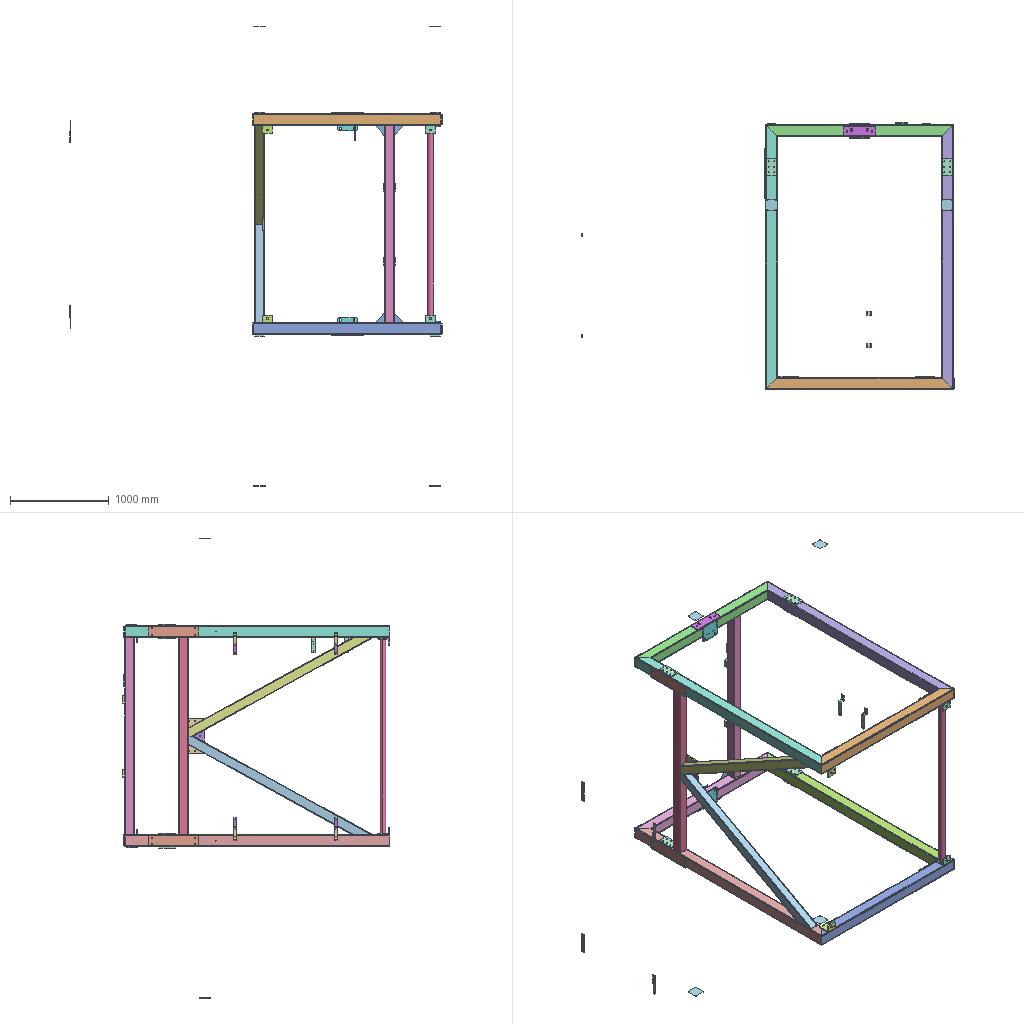Assembly | SolidWorks | 34 different items | 72 placed | box 3771 x 2705 x 4658 mm
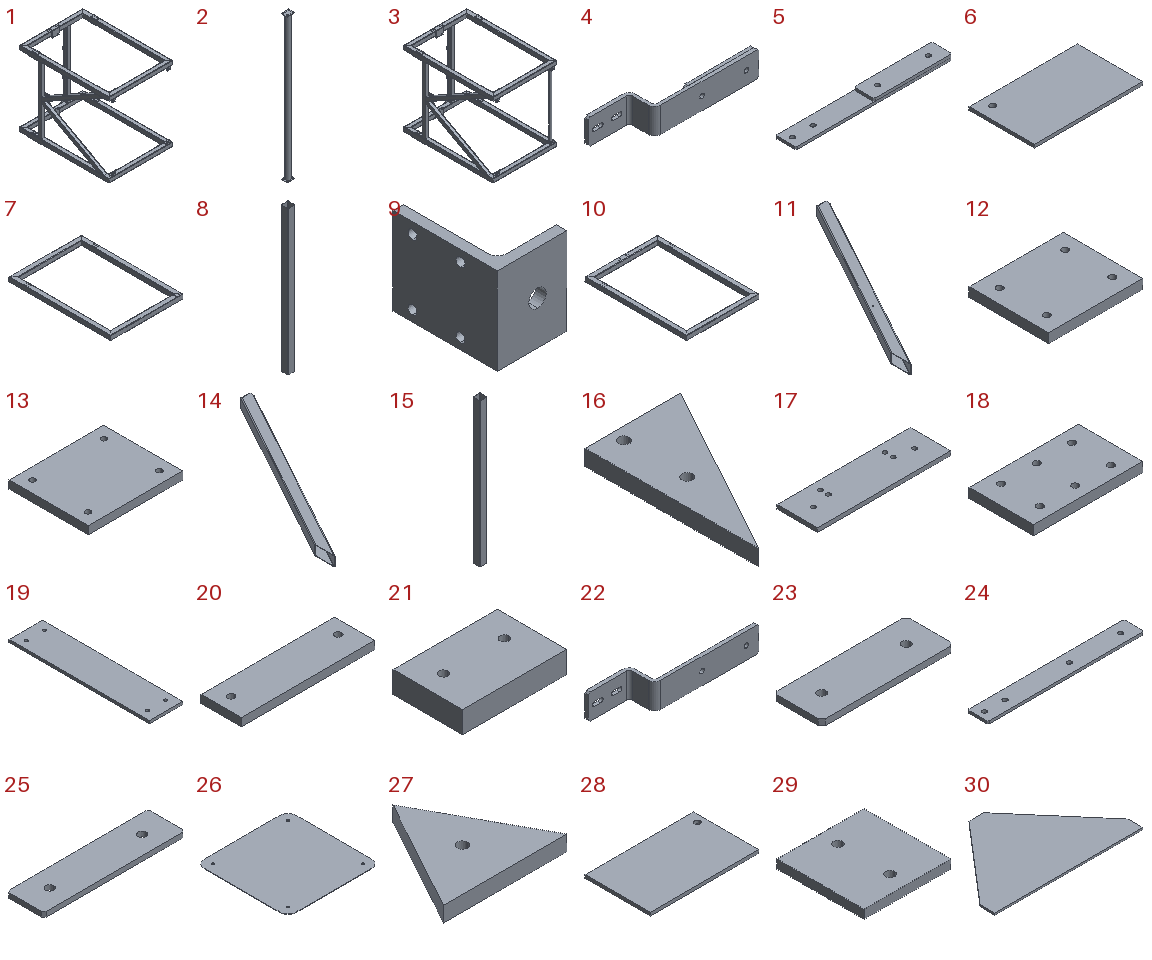Parts list (item | name | quantity | parent item | size | volume | features):
1 | (subassembly) | x1 | in 3 | 1920 x 2705 x 2270 mm | 51706109 mm3 | features CompositeCurve 25
2 | (subassembly) | x1 | in 3 | 100 x 80 x 1976 mm | 1280209 mm3 | -
3 | (subassembly) | x1 | - | 1920 x 2705 x 2270 mm | 52986318 mm3 | features CompositeCurve 4
4 | (subassembly) | x2 | - | 230 x 45 x 40 mm | 72678 mm3 | -
5 | (subassembly) | x4 | - | 230 x 30 x 8 mm | 40540 mm3 | features CompositeCurve 1
6 | - | x2 | in 1 | 200 x 120 x 6 mm | 143510 mm3 | features Extrusion 1, HoleWzd 1
7 | - | x1 | in 1 | 1900 x 2680 x 120 mm | 15591720 mm3 | features ICE 8, HoleWzd 6, 3DProfileFeature 1, WeldMemberFeat 1, WeldmentFeature 1
8 | - | x1 | in 1 | 100 x 100 x 2000 mm | 2980690 mm3 | features Extrusion 1, Fillet 1, HoleWzd 1, ICE 1, Shell 1
9 | - | x2 | in 1 | 80 x 120 x 100 mm | 220054 mm3 | features Extrusion 1, HoleWzd 1, ICE 1
10 | - | x1 | in 1 | 1900 x 2680 x 120 mm | 15602458 mm3 | features HoleWzd 7, ICE 7, WeldMemberFeat 1, WeldmentFeature 1
11 | - | x1 | in 1 | 1000 x 1874 x 100 mm | 3026106 mm3 | features Fillet 2, Extrusion 1, HoleWzd 1, Shell 1
12 | - | x4 | in 1 | 100 x 85 x 10 mm | 83547 mm3 | features Extrusion 1, HoleWzd 1
13 | - | x1 | in 1 | 120 x 100 x 10 mm | 118547 mm3 | features Extrusion 1, HoleWzd 1
14 | - | x1 | in 1 | 1000 x 1874 x 100 mm | 3026106 mm3 | features Fillet 2, Extrusion 1, HoleWzd 1, Shell 1
15 | - | x1 | in 1 | 100 x 100 x 2000 mm | 2986846 mm3 | features Extrusion 1, Shell 1
16 | - | x2 | in 1 | 90.635 x 165 x 15 mm | 109709 mm3 | features Extrusion 1, HoleWzd 1
17 | - | x2 | in 1 | 330 x 100 x 10 mm | 325097 mm3 | features Extrusion 1, HoleWzd 1
18 | - | x8 | in 1 | 170 x 100 x 15 mm | 247646 mm3 | features Extrusion 1, HoleWzd 1
19 | - | x2 | in 1 | 120 x 505 x 10 mm | 602731 mm3 | features Extrusion 1, HoleWzd 1
20 | - | x2 | in 1 | 200 x 60 x 12 mm | 142039 mm3 | features Extrusion 1, HoleWzd 1
21 | - | x2 | in 1 | 120 x 80 x 25 mm | 235914 mm3 | features Extrusion 1, HoleWzd 1
22 | - | x2 | in 4 | 230 x 45 x 40 mm | 51153 mm3 | features ICE 2, Chamfer 1, Extrusion 1
23 | - | x2 | in 4 | 110 x 40 x 5 mm | 21525 mm3 | features Chamfer 1, Extrusion 1
24 | - | x4 | in 5 | 230 x 30 x 4 mm | 27037 mm3 | features Chamfer 1, Extrusion 1
25 | - | x4 | in 5 | 115 x 30 x 4 mm | 13503 mm3 | features Chamfer 1, Extrusion 1
26 | - | x4 | - | 115 x 115 x 0.5 mm | 6555 mm3 | features Extrusion 1
27 | - | x1 | in 1 | 121 x 110.14 x 15 mm | 98726 mm3 | features Extrusion 1, HoleWzd 1
28 | - | x2 | in 1 | 200 x 120 x 6 mm | 143510 mm3 | features Extrusion 1, HoleWzd 1
29 | - | x2 | in 1 | 100 x 100 x 10 mm | 98366 mm3 | features Extrusion 1, HoleWzd 1
30 | - | x2 | in 1 | 400 x 250 x 5 mm | 311000 mm3 | features Extrusion 1, ICE 1
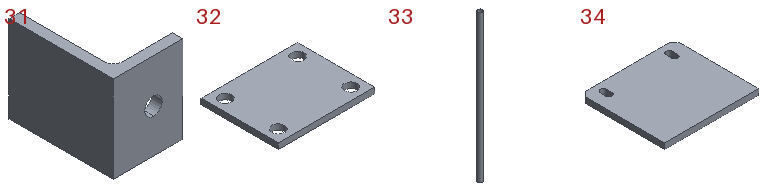31 | - | x2 | in 1 | 80 x 120 x 100 mm | 223976 mm3 | features Extrusion 1, ICE 1
32 | - | x2 | in 2 | 100 x 80 x 6 mm | 44814 mm3 | features Extrusion 1, ICE 1
33 | - | x1 | in 2 | 63.5 x 63.5 x 1964 mm | 1190580 mm3 | features Extrusion 1, Shell 1
34 | - | x2 | in 1 | 200 x 180 x 12 mm | 423870 mm3 | features Chamfer 1, Extrusion 1, ICE 1
Mates (type | each side: item.copy, entity, surface, feature):
In the top assembly
Coincident | 7.1 face plane Rectangular Tube 120 X 80 X 8(1) | 26.1 face plane Boss-Extrude1
Concentric | 7.1 edge | 26.1 edge
Coincident | 7.1 face cylinder Cut-Extrude1 | 26.1 edge
Coincident | 26.2 face plane Boss-Extrude1 | 26.1 face plane Boss-Extrude1
Coincident | 7.1 face cylinder Cut-Extrude1 | 26.2 edge
Concentric | 7.1 face cylinder Cut-Extrude1 | 26.2 face cylinder Boss-Extrude1
Coincident | 10.1 face plane Rectangular Tube 120 X 80 X 8(1) | 26.3 face plane Boss-Extrude1
Coincident | 10.1 face plane Rectangular Tube 120 X 80 X 8(1) | 26.4 face plane Boss-Extrude1
Concentric | 10.1 face cylinder Cut-Extrude5 | 26.4 face cylinder Boss-Extrude1 | 2 times
Concentric | 10.1 face cylinder Cut-Extrude5 | 26.3 face cylinder Boss-Extrude1 | 2 times
Coincident | 10.1 face plane Rectangular Tube 120 X 80 X 8(1) | 24.1 face plane Boss-Extrude1
Concentric | 10.1 edge | 24.1 edge | 2 times
Coincident | 10.1 face plane Rectangular Tube 120 X 80 X 8(1) | 24.2 face plane Boss-Extrude1
Concentric | 10.1 face cylinder M6 Tapped Hole1 | 24.2 face cylinder Boss-Extrude1 | 2 times
Coincident | 7.1 face plane Rectangular Tube 120 X 80 X 8(1) | 24.3 face plane Boss-Extrude1
Concentric | 7.1 face cylinder M6 Tapped Hole1 | 24.3 edge
Concentric | 7.1 face cylinder M6 Tapped Hole1 | 24.3 face cylinder Boss-Extrude1
Coincident | 7.1 face plane Rectangular Tube 120 X 80 X 8(1) | 24.4 face plane Boss-Extrude1
Concentric | 7.1 face cylinder M6 Tapped Hole1 | 24.4 face cylinder Boss-Extrude1
Concentric | 7.1 edge | 24.4 face cylinder Boss-Extrude1
Coincident | 10.1 face plane Rectangular Tube 120 X 80 X 8(1) | 22.1 face plane Boss-Extrude1
Parallel | 10.1 face plane Rectangular Tube 120 X 80 X 8(1) | 22.1 face plane Boss-Extrude1
Coincident | 10.1 face plane Rectangular Tube 120 X 80 X 8(1) | 22.2 face plane Boss-Extrude1
Coincident | 22.1 face plane Boss-Extrude1 | 22.2 face plane Boss-Extrude1
In subassembly 4
Coincident | 22.3 face plane Boss-Extrude1 | 23.1 face plane Boss-Extrude1
Concentric | 22.3 face cylinder Cut-Extrude2 | 23.1 face cylinder Boss-Extrude1 | 2 times
In subassembly 5
Coincident | 24.5 face plane Boss-Extrude1 | 25.1 face plane Boss-Extrude1
Coincident | 24.5 edge | 25.1 face cylinder Boss-Extrude1
Concentric | 24.5 face cylinder Boss-Extrude1 | 25.1 face cylinder Boss-Extrude1
In subassembly 3
Coincident | 9.1 face plane Boss-Extrude1 | 32.1 face plane Boss-Extrude1
Concentric | 9.1 select_type:24 | 32.1 edge
Concentric | 9.1 edge | 32.1 edge
In subassembly 2
Coincident | 32.2 face plane Boss-Extrude1 | 33.1 face plane Boss-Extrude1
Coincident | 32.2 plane | 33.1 plane | 2 times
Coincident | 32.2 face plane Boss-Extrude1 | 32.3 face plane Boss-Extrude1 | 2 times
Coincident | 33.1 face plane Boss-Extrude1 | 32.3 face plane Boss-Extrude1
In subassembly 1
Coincident | 7.2 face plane Rectangular Tube 120 X 80 X 8(1) | 10.2 face plane Rectangular Tube 120 X 80 X 8(1) | 2 times
Coincident | 7.2 face plane Rectangular Tube 120 X 80 X 8(1) | 15.1 face plane Boss-Extrude1
Coincident | 10.2 face plane Rectangular Tube 120 X 80 X 8(1) | 15.1 face plane Boss-Extrude1
DistanceDim | 15.1 face plane Boss-Extrude1 | 7.2 face plane Rectangular Tube 120 X 80 X 8(1)
Width | 7.2 face plane Rectangular Tube 120 X 80 X 8(1) | 7.2 face plane Rectangular Tube 120 X 80 X 8(1) | 15.1 face plane Boss-Extrude1 | 15.1 face plane Boss-Extrude1
Coincident | 7.2 face plane Rectangular Tube 120 X 80 X 8(1) | 14.1 face plane Boss-Extrude1
Width | 14.1 face plane Boss-Extrude1 | 14.1 face plane Boss-Extrude1 | 7.2 face plane Rectangular Tube 120 X 80 X 8(1) | 7.2 face plane Rectangular Tube 120 X 80 X 8(1)
Coincident | 15.1 face plane Boss-Extrude1 | 14.1 face plane Boss-Extrude1
Coincident | 10.2 face plane Rectangular Tube 120 X 80 X 8(1) | 11.1 face plane Boss-Extrude1
Coincident | 14.1 face plane Boss-Extrude1 | 11.1 face plane Boss-Extrude1 | 2 times
Coincident | 15.1 face plane Boss-Extrude1 | 11.1 face plane Boss-Extrude1
Coincident | 10.2 face plane Rectangular Tube 120 X 80 X 8(1) | 17.1 face plane Boss-Extrude1
Concentric | 10.2 edge | 17.1 edge | 2 times
Coincident | 7.2 face plane Rectangular Tube 120 X 80 X 8(1) | 17.2 face plane Boss-Extrude1
Concentric | 7.2 edge | 17.2 face cylinder M12 Tapped Hole1
Concentric | 7.2 edge | 17.2 edge
Coincident | 7.2 face plane Rectangular Tube 120 X 80 X 8(1) | 18.1 face plane Boss-Extrude1
Concentric | 7.2 edge | 18.1 edge | 2 times
Coincident | 7.2 face plane Rectangular Tube 120 X 80 X 8(1) | 18.2 face plane Boss-Extrude1
Concentric | 7.2 edge | 18.2 edge | 2 times
Concentric | 7.2 face cylinder Cut-Extrude2 | 18.3 face cylinder M12 Tapped Hole1 | 2 times
Coincident | 7.2 face plane Rectangular Tube 120 X 80 X 8(1) | 18.3 face plane Boss-Extrude1
Coincident | 7.2 face plane Rectangular Tube 120 X 80 X 8(1) | 18.4 face plane Boss-Extrude1
Concentric | 7.2 edge | 19.1 edge | 2 times
Coincident | 19.1 face plane Boss-Extrude1 | 19.2 face plane Boss-Extrude1
Concentric | 10.2 face cylinder M12 Tapped Hole1 | 19.2 face cylinder M12 Tapped Hole1 | 2 times
Coincident | 7.2 face plane Rectangular Tube 120 X 80 X 8(1) | 19.1 face plane Boss-Extrude1
Coincident | 7.2 face plane Rectangular Tube 120 X 80 X 8(1) | 20.1 face plane Boss-Extrude1
Concentric | 7.2 face cylinder Cut-Extrude10 | 20.1 face cylinder M12 Tapped Hole1 | 2 times
Coincident | 10.2 face plane Rectangular Tube 120 X 80 X 8(1) | 20.2 face plane Boss-Extrude1
Concentric | 10.2 face cylinder Cut-Extrude7 | 20.2 face cylinder M12 Tapped Hole1 | 2 times
Coincident | 7.2 face plane Rectangular Tube 120 X 80 X 8(1) | 8.1 face plane Boss-Extrude1 | 2 times
DistanceDim | 8.1 face plane Boss-Extrude1 | 10.2 face plane Rectangular Tube 120 X 80 X 8(1)
Coincident | 21.1 face plane Boss-Extrude1 | 21.2 face plane Boss-Extrude1
Coincident | 21.2 face plane Boss-Extrude1 | 8.1 face plane Boss-Extrude1
Coincident | 10.2 face plane Rectangular Tube 120 X 80 X 8(1) | 34.1 face plane Boss-Extrude1
DistanceDim | 34.1 face plane Boss-Extrude1 | 10.2 face plane Rectangular Tube 120 X 80 X 8(1)
Width | 34.1 face plane Boss-Extrude1 | 34.1 face plane Boss-Extrude1 | 20.2 face plane Boss-Extrude1 | 20.2 face plane Boss-Extrude1
Coincident | 34.1 face plane Boss-Extrude1 | 34.2 face plane Boss-Extrude1
Coincident | 7.2 face plane Rectangular Tube 120 X 80 X 8(1) | 34.2 face plane Boss-Extrude1
DistanceDim | 34.2 face plane Boss-Extrude1 | 7.2 face plane Rectangular Tube 120 X 80 X 8(1)
Parallel | 11.1 face plane Boss-Extrude1 | 27.1 face plane Boss-Extrude1
Coincident | 11.1 face plane Boss-Extrude1 | 27.1 face plane Boss-Extrude1
Coincident | 11.1 edge | 27.1 edge
Coincident | 14.1 face plane Boss-Extrude1 | 27.1 face plane Boss-Extrude1
Coincident | 15.1 face plane Boss-Extrude1 | 16.1 face plane Boss-Extrude2
Coincident | 11.1 edge | 16.1 edge
Coincident | 27.1 face plane Boss-Extrude1 | 16.1 face plane Boss-Extrude2
Coincident | 16.2 face plane Boss-Extrude2 | 16.1 face plane Boss-Extrude2
Coincident | 15.1 face plane Boss-Extrude1 | 16.2 face plane Boss-Extrude2
Coincident | 14.1 edge | 16.2 edge
Coincident | 10.2 face plane Rectangular Tube 120 X 80 X 8(1) | 28.1 face plane Boss-Extrude1
Concentric | 10.2 face cylinder Cut-Extrude6 | 28.1 face cylinder M12 Tapped Hole1
Parallel | 10.2 face plane Rectangular Tube 120 X 80 X 8(1) | 28.1 face plane Boss-Extrude1
Concentric | 7.2 face cylinder Cut-Extrude9 | 28.2 face cylinder M12 Tapped Hole1
Coincident | 7.2 face plane Rectangular Tube 120 X 80 X 8(1) | 28.2 face plane Boss-Extrude1
Parallel | 7.2 face plane Rectangular Tube 120 X 80 X 8(1) | 28.2 face plane Boss-Extrude1
Coincident | 10.2 face plane Rectangular Tube 120 X 80 X 8(1) | 29.1 face plane Boss-Extrude1
Concentric | 10.2 edge | 29.1 face cylinder M12 Tapped Hole1
Concentric | 10.2 edge | 29.1 edge
Coincident | 7.2 face plane Rectangular Tube 120 X 80 X 8(1) | 29.2 face plane Boss-Extrude1
Concentric | 7.2 edge | 29.2 face cylinder M12 Tapped Hole1
Concentric | 7.2 face cylinder Cut-Extrude5 | 29.2 edge
Coincident | 10.2 face plane Rectangular Tube 120 X 80 X 8(1) | 30.1 face plane Boss-Extrude1
Coincident | 10.2 edge | 30.1 face plane Boss-Extrude1
Width | 30.1 face plane Cut-Extrude1 | 30.1 face plane Cut-Extrude1 | 8.1 face plane Boss-Extrude1 | 8.1 face plane Boss-Extrude1
Coincident | 7.2 face plane Rectangular Tube 120 X 80 X 8(1) | 30.2 face plane Boss-Extrude1
Coincident | 7.2 edge | 30.2 face plane Boss-Extrude1
Coincident | 30.1 face plane Boss-Extrude1 | 30.2 face plane Boss-Extrude1
Coincident | 10.2 face plane Rectangular Tube 120 X 80 X 8(1) | 31.1 face plane Boss-Extrude1 | 2 times
Coincident | 7.2 face plane Rectangular Tube 120 X 80 X 8(1) | 31.2 face plane Boss-Extrude1 | 2 times
Concentric | 7.2 face cylinder Cut-Extrude9 | 6.1 face cylinder M12 Tapped Hole1
Coincident | 7.2 face plane Rectangular Tube 120 X 80 X 8(1) | 6.1 face plane Boss-Extrude1
Parallel | 7.2 face plane Rectangular Tube 120 X 80 X 8(1) | 6.1 face plane Boss-Extrude1
Coincident | 10.2 face plane Rectangular Tube 120 X 80 X 8(1) | 6.2 face plane Boss-Extrude1
Concentric | 10.2 face cylinder Cut-Extrude6 | 6.2 face cylinder M12 Tapped Hole1
Parallel | 10.2 face plane Rectangular Tube 120 X 80 X 8(1) | 6.2 face plane Boss-Extrude1
Coincident | 10.2 face plane Rectangular Tube 120 X 80 X 8(1) | 9.2 face plane Boss-Extrude1
Concentric | 10.2 face cylinder Cut-Extrude9 | 9.2 face cylinder M12 Tapped Hole1 | 2 times
Coincident | 7.2 face plane Rectangular Tube 120 X 80 X 8(1) | 9.3 face plane Boss-Extrude1
Concentric | 7.2 face cylinder Cut-Extrude12 | 9.3 face cylinder M12 Tapped Hole1 | 2 times
Coincident | 10.2 face plane Rectangular Tube 120 X 80 X 8(1) | 12.1 face plane Boss-Extrude1
Concentric | 10.2 face cylinder Cut-Extrude7 | 12.1 face cylinder M8 Tapped Hole1 | 2 times
Coincident | 12.2 face plane Boss-Extrude1 | 12.3 face plane Boss-Extrude1
Coincident | 12.4 face plane Boss-Extrude1 | 12.3 face plane Boss-Extrude1
Coincident | 12.1 face plane Boss-Extrude1 | 12.4 face plane Boss-Extrude1
Concentric | 10.2 face cylinder Cut-Extrude7 | 12.4 face cylinder M8 Tapped Hole1 | 2 times
Concentric | 7.2 face cylinder Cut-Extrude10 | 12.3 face cylinder M8 Tapped Hole1 | 2 times
Concentric | 7.2 face cylinder Cut-Extrude10 | 12.2 face cylinder M8 Tapped Hole1 | 2 times
Coincident | 8.1 face plane Boss-Extrude1 | 13.1 face plane Boss-Extrude1
Concentric | 8.1 face cylinder M8 Tapped Hole1 | 13.1 face cylinder M8 Tapped Hole1 | 2 times
Coincident | 21.1 face plane Boss-Extrude1 | 8.1 face plane Boss-Extrude1
Concentric | 21.1 face cylinder M12 Tapped Hole1 | 8.1 face cylinder Cut-Extrude1 | 2 times
Concentric | 21.2 face cylinder M12 Tapped Hole1 | 8.1 face cylinder Cut-Extrude1 | 2 times
Concentric | 10.2 face cylinder Cut-Extrude2 | 18.5 face cylinder M12 Tapped Hole1 | 2 times
Coincident | 10.2 face plane Rectangular Tube 120 X 80 X 8(1) | 18.5 face plane Boss-Extrude1
Concentric | 10.2 face cylinder Cut-Extrude2 | 18.6 face cylinder M12 Tapped Hole1 | 2 times
Coincident | 10.2 face plane Rectangular Tube 120 X 80 X 8(1) | 18.6 face plane Boss-Extrude1
Concentric | 10.2 face cylinder Cut-Extrude2 | 18.7 face cylinder M12 Tapped Hole1 | 2 times
Concentric | 10.2 face cylinder Cut-Extrude2 | 18.8 face cylinder M12 Tapped Hole1 | 2 times
Concentric | 7.2 face cylinder Cut-Extrude2 | 18.4 face cylinder M12 Tapped Hole1 | 2 times
Coincident | 31.1 face plane Boss-Extrude1 | 31.2 face plane Boss-Extrude1
DistanceDim | 31.1 face plane Boss-Extrude1 | 10.2 face plane Rectangular Tube 120 X 80 X 8(1)